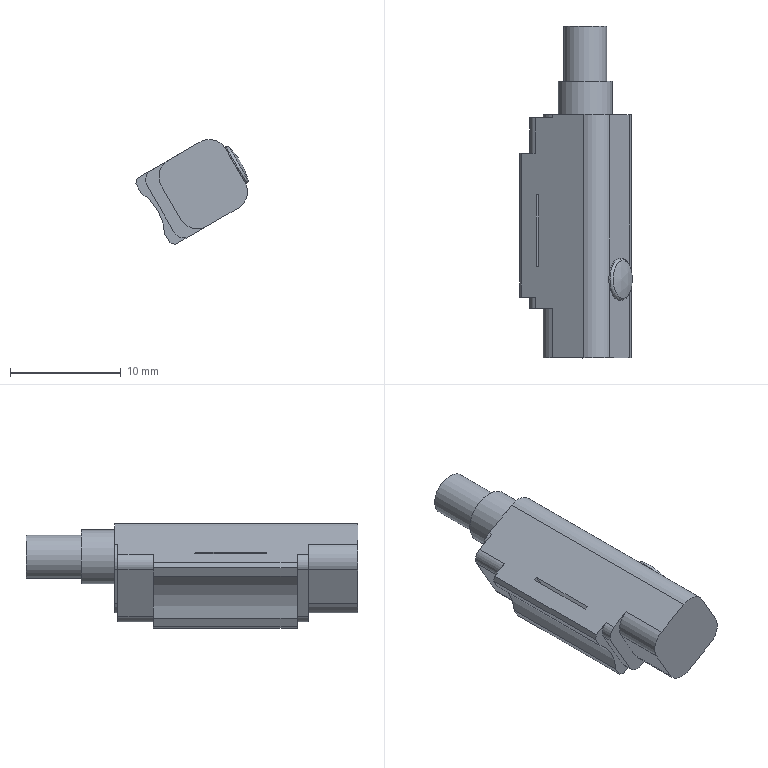Part | NX | features WGN01-25-100-Y-2-003 2 | 1 solid | 42 faces | box 10.179 x 30 x 9.481 mm | volume 1272 mm3 | plane 26 | cylinder 14 | torus 1 | sphere 1 | commonest cylinder face diameters 3.4 x6 2 x4 3.8 x1 3.9 x1 4.9 x1 10 x1
STEP:
#1=CARTESIAN_POINT('',(19.571,368.576,148.202));
#2=VERTEX_POINT('',#1);
#3=CARTESIAN_POINT('',(19.571,370.056,148.202));
#4=VERTEX_POINT('',#3);
#5=CARTESIAN_POINT('',(20.446,369.316,146.686));
#6=DIRECTION('',(-0.866,0.,-0.5));
#7=DIRECTION('',(-0.4605,-0.3894,0.7977));
#8=AXIS2_PLACEMENT_3D('',#5,#6,#7);
#9=CIRCLE('',#8,1.9);
#10=EDGE_CURVE('',#2,#4,#9,.T.);
#11=ORIENTED_EDGE('',*,*,#10,.F.);
#12=CARTESIAN_POINT('',(21.321,368.576,145.17));
#13=VERTEX_POINT('',#12);
#14=CARTESIAN_POINT('',(20.446,369.316,146.686));
#15=DIRECTION('',(-0.866,0.,-0.5));
#16=DIRECTION('',(0.4605,-0.3894,-0.7977));
#17=AXIS2_PLACEMENT_3D('',#14,#15,#16);
#18=CIRCLE('',#17,1.9);
#19=EDGE_CURVE('',#13,#2,#18,.T.);
#20=ORIENTED_EDGE('',*,*,#19,.F.);
#21=CARTESIAN_POINT('',(21.321,370.056,145.17));
#22=VERTEX_POINT('',#21);
#23=CARTESIAN_POINT('',(20.446,369.316,146.686));
#24=DIRECTION('',(-0.866,0.,-0.5));
#25=DIRECTION('',(0.4605,0.3894,-0.7977));
#26=AXIS2_PLACEMENT_3D('',#23,#24,#25);
#27=CIRCLE('',#26,1.9);
#28=EDGE_CURVE('',#22,#13,#27,.T.);
#29=ORIENTED_EDGE('',*,*,#28,.F.);
#30=CARTESIAN_POINT('',(20.446,369.316,146.686));
#31=DIRECTION('',(-0.866,0.,-0.5));
#32=DIRECTION('',(-0.4605,0.3894,0.7977));
#33=AXIS2_PLACEMENT_3D('',#30,#31,#32);
#34=CIRCLE('',#33,1.9);
#35=EDGE_CURVE('',#4,#22,#34,.T.);
#36=ORIENTED_EDGE('',*,*,#35,.F.);
#37=EDGE_LOOP('',(#11,#20,#29,#36));
#38=FACE_BOUND('',#37,.T.);
#39=CARTESIAN_POINT('',(19.596,369.316,148.389));
#40=VERTEX_POINT('',#39);
#41=CARTESIAN_POINT('',(20.546,369.316,146.744));
#42=DIRECTION('',(-0.866,0.,-0.5));
#43=DIRECTION('',(-0.5,0.,0.866));
#44=AXIS2_PLACEMENT_3D('',#41,#42,#43);
#45=CIRCLE('',#44,1.9);
#46=EDGE_CURVE('',#40,#40,#45,.T.);
#47=ORIENTED_EDGE('',*,*,#46,.T.);
#48=EDGE_LOOP('',(#47));
#49=FACE_BOUND('',#48,.T.);
#50=CARTESIAN_POINT('',(20.446,369.316,146.686));
#51=DIRECTION('',(-0.866,0.,-0.5));
#52=DIRECTION('',(0.5,0.,-0.866));
#53=AXIS2_PLACEMENT_3D('',#50,#51,#52);
#54=CYLINDRICAL_SURFACE('',#53,1.9);
#55=ADVANCED_FACE('',(#38,#49),#54,.T.);
#56=ORIENTED_EDGE('',*,*,#46,.F.);
#57=EDGE_LOOP('',(#56));
#58=FACE_BOUND('',#57,.T.);
#59=CARTESIAN_POINT('',(19.894,369.316,148.353));
#60=VERTEX_POINT('',#59);
#61=CARTESIAN_POINT('',(20.754,369.316,146.864));
#62=DIRECTION('',(-0.866,0.,-0.5));
#63=DIRECTION('',(-0.5,0.,0.866));
#64=AXIS2_PLACEMENT_3D('',#61,#62,#63);
#65=CIRCLE('',#64,1.72);
#66=EDGE_CURVE('',#60,#60,#65,.T.);
#67=ORIENTED_EDGE('',*,*,#66,.T.);
#68=EDGE_LOOP('',(#67));
#69=FACE_BOUND('',#68,.T.);
#70=CARTESIAN_POINT('',(20.546,369.316,146.744));
#71=DIRECTION('',(-0.866,0.,-0.5));
#72=DIRECTION('',(0.5,0.,-0.866));
#73=AXIS2_PLACEMENT_3D('',#70,#71,#72);
#74=TOROIDAL_SURFACE('',#73,1.65,0.25);
#75=ADVANCED_FACE('',(#58,#69),#74,.T.);
#76=ORIENTED_EDGE('',*,*,#66,.F.);
#77=EDGE_LOOP('',(#76));
#78=FACE_BOUND('',#77,.T.);
#79=CARTESIAN_POINT('',(15.623,369.316,143.901));
#80=DIRECTION('',(0.5,0.,-0.866));
#81=DIRECTION('',(0.,-1.,0.));
#82=AXIS2_PLACEMENT_3D('',#79,#80,#81);
#83=SPHERICAL_SURFACE('',#82,6.17);
#84=ADVANCED_FACE('',(#78),#83,.T.);
#85=CARTESIAN_POINT('',(18.323,387.216,144.363));
#86=VERTEX_POINT('',#85);
#87=CARTESIAN_POINT('',(17.348,387.216,146.052));
#88=DIRECTION('',(0.,-1.,0.));
#89=DIRECTION('',(0.5,0.,-0.866));
#90=AXIS2_PLACEMENT_3D('',#87,#88,#89);
#91=CIRCLE('',#90,1.95);
#92=EDGE_CURVE('',#86,#86,#91,.F.);
#93=ORIENTED_EDGE('',*,*,#92,.T.);
#94=EDGE_LOOP('',(#93));
#95=FACE_BOUND('',#94,.T.);
#96=CARTESIAN_POINT('',(18.323,392.216,144.363));
#97=VERTEX_POINT('',#96);
#98=CARTESIAN_POINT('',(17.348,392.216,146.052));
#99=DIRECTION('',(0.,-1.,0.));
#100=DIRECTION('',(0.5,0.,-0.866));
#101=AXIS2_PLACEMENT_3D('',#98,#99,#100);
#102=CIRCLE('',#101,1.95);
#103=EDGE_CURVE('',#97,#97,#102,.F.);
#104=ORIENTED_EDGE('',*,*,#103,.F.);
#105=EDGE_LOOP('',(#104));
#106=FACE_BOUND('',#105,.T.);
#107=CARTESIAN_POINT('',(17.348,392.216,146.052));
#108=DIRECTION('',(0.,-1.,0.));
#109=DIRECTION('',(-0.5,0.,0.866));
#110=AXIS2_PLACEMENT_3D('',#107,#108,#109);
#111=CYLINDRICAL_SURFACE('',#110,1.95);
#112=ADVANCED_FACE('',(#95,#106),#111,.T.);
#113=CARTESIAN_POINT('',(16.123,384.216,148.174));
#114=VERTEX_POINT('',#113);
#115=CARTESIAN_POINT('',(17.348,384.216,146.052));
#116=DIRECTION('',(0.,-1.,0.));
#117=DIRECTION('',(0.5,0.,-0.866));
#118=AXIS2_PLACEMENT_3D('',#115,#116,#117);
#119=CIRCLE('',#118,2.45);
#120=EDGE_CURVE('',#114,#114,#119,.F.);
#121=ORIENTED_EDGE('',*,*,#120,.T.);
#122=EDGE_LOOP('',(#121));
#123=FACE_BOUND('',#122,.T.);
#124=CARTESIAN_POINT('',(18.573,387.216,143.93));
#125=VERTEX_POINT('',#124);
#126=CARTESIAN_POINT('',(17.348,387.216,146.052));
#127=DIRECTION('',(0.,-1.,0.));
#128=DIRECTION('',(0.5,0.,-0.866));
#129=AXIS2_PLACEMENT_3D('',#126,#127,#128);
#130=CIRCLE('',#129,2.45);
#131=EDGE_CURVE('',#125,#125,#130,.F.);
#132=ORIENTED_EDGE('',*,*,#131,.F.);
#133=EDGE_LOOP('',(#132));
#134=FACE_BOUND('',#133,.T.);
#135=CARTESIAN_POINT('',(17.348,387.216,146.052));
#136=DIRECTION('',(0.,-1.,0.));
#137=DIRECTION('',(-0.5,0.,0.866));
#138=AXIS2_PLACEMENT_3D('',#135,#136,#137);
#139=CYLINDRICAL_SURFACE('',#138,2.45);
#140=ADVANCED_FACE('',(#123,#134),#139,.T.);
#141=CARTESIAN_POINT('',(20.699,384.216,142.848));
#142=VERTEX_POINT('',#141);
#143=CARTESIAN_POINT('',(20.699,362.216,142.848));
#144=VERTEX_POINT('',#143);
#145=CARTESIAN_POINT('',(20.699,384.216,142.848));
#146=DIRECTION('',(0.,-1.,0.));
#147=VECTOR('',#146,1000.);
#148=LINE('',#145,#147);
#149=EDGE_CURVE('',#142,#144,#148,.T.);
#150=ORIENTED_EDGE('',*,*,#149,.T.);
#151=CARTESIAN_POINT('',(17.841,362.216,141.198));
#152=VERTEX_POINT('',#151);
#153=CARTESIAN_POINT('',(20.699,362.216,142.848));
#154=DIRECTION('',(-0.866,0.,-0.5));
#155=VECTOR('',#154,1000.);
#156=LINE('',#153,#155);
#157=EDGE_CURVE('',#144,#152,#156,.T.);
#158=ORIENTED_EDGE('',*,*,#157,.T.);
#159=CARTESIAN_POINT('',(17.841,366.716,141.198));
#160=VERTEX_POINT('',#159);
#161=CARTESIAN_POINT('',(17.841,366.716,141.198));
#162=DIRECTION('',(0.,-1.,0.));
#163=VECTOR('',#162,1000.);
#164=LINE('',#161,#163);
#165=EDGE_CURVE('',#160,#152,#164,.T.);
#166=ORIENTED_EDGE('',*,*,#165,.F.);
#167=CARTESIAN_POINT('',(16.282,366.716,140.298));
#168=VERTEX_POINT('',#167);
#169=CARTESIAN_POINT('',(17.841,366.716,141.198));
#170=DIRECTION('',(-0.866,0.,-0.5));
#171=VECTOR('',#170,1000.);
#172=LINE('',#169,#171);
#173=EDGE_CURVE('',#160,#168,#172,.T.);
#174=ORIENTED_EDGE('',*,*,#173,.T.);
#175=CARTESIAN_POINT('',(16.282,367.716,140.298));
#176=VERTEX_POINT('',#175);
#177=CARTESIAN_POINT('',(16.282,367.716,140.298));
#178=DIRECTION('',(0.,-1.,0.));
#179=VECTOR('',#178,1000.);
#180=LINE('',#177,#179);
#181=EDGE_CURVE('',#176,#168,#180,.T.);
#182=ORIENTED_EDGE('',*,*,#181,.F.);
#183=CARTESIAN_POINT('',(15.021,367.716,139.57));
#184=VERTEX_POINT('',#183);
#185=CARTESIAN_POINT('',(16.282,367.716,140.298));
#186=DIRECTION('',(-0.866,0.,-0.5));
#187=VECTOR('',#186,1000.);
#188=LINE('',#185,#187);
#189=EDGE_CURVE('',#176,#184,#188,.T.);
#190=ORIENTED_EDGE('',*,*,#189,.T.);
#191=CARTESIAN_POINT('',(15.021,380.716,139.57));
#192=VERTEX_POINT('',#191);
#193=CARTESIAN_POINT('',(15.021,380.716,139.57));
#194=DIRECTION('',(0.,-1.,0.));
#195=VECTOR('',#194,1000.);
#196=LINE('',#193,#195);
#197=EDGE_CURVE('',#192,#184,#196,.T.);
#198=ORIENTED_EDGE('',*,*,#197,.F.);
#199=CARTESIAN_POINT('',(16.282,380.716,140.298));
#200=VERTEX_POINT('',#199);
#201=CARTESIAN_POINT('',(16.282,380.716,140.298));
#202=DIRECTION('',(-0.866,0.,-0.5));
#203=VECTOR('',#202,1000.);
#204=LINE('',#201,#203);
#205=EDGE_CURVE('',#200,#192,#204,.T.);
#206=ORIENTED_EDGE('',*,*,#205,.F.);
#207=CARTESIAN_POINT('',(16.282,383.916,140.298));
#208=VERTEX_POINT('',#207);
#209=CARTESIAN_POINT('',(16.282,383.916,140.298));
#210=DIRECTION('',(0.,-1.,0.));
#211=VECTOR('',#210,1000.);
#212=LINE('',#209,#211);
#213=EDGE_CURVE('',#208,#200,#212,.T.);
#214=ORIENTED_EDGE('',*,*,#213,.F.);
#215=CARTESIAN_POINT('',(17.841,383.916,141.198));
#216=VERTEX_POINT('',#215);
#217=CARTESIAN_POINT('',(17.841,383.916,141.198));
#218=DIRECTION('',(-0.866,0.,-0.5));
#219=VECTOR('',#218,1000.);
#220=LINE('',#217,#219);
#221=EDGE_CURVE('',#216,#208,#220,.T.);
#222=ORIENTED_EDGE('',*,*,#221,.F.);
#223=CARTESIAN_POINT('',(17.841,384.216,141.198));
#224=VERTEX_POINT('',#223);
#225=CARTESIAN_POINT('',(17.841,384.216,141.198));
#226=DIRECTION('',(0.,-1.,0.));
#227=VECTOR('',#226,1000.);
#228=LINE('',#225,#227);
#229=EDGE_CURVE('',#224,#216,#228,.T.);
#230=ORIENTED_EDGE('',*,*,#229,.F.);
#231=CARTESIAN_POINT('',(20.699,384.216,142.848));
#232=DIRECTION('',(-0.866,0.,-0.5));
#233=VECTOR('',#232,1000.);
#234=LINE('',#231,#233);
#235=EDGE_CURVE('',#142,#224,#234,.T.);
#236=ORIENTED_EDGE('',*,*,#235,.F.);
#237=EDGE_LOOP('',(#150,#158,#166,#174,#182,#190,#198,#206,#214,#222,#230,#236));
#238=FACE_BOUND('',#237,.T.);
#239=CARTESIAN_POINT('',(16.629,376.966,140.498));
#240=VERTEX_POINT('',#239);
#241=CARTESIAN_POINT('',(16.629,370.466,140.498));
#242=VERTEX_POINT('',#241);
#243=CARTESIAN_POINT('',(16.629,376.966,140.498));
#244=DIRECTION('',(0.,-1.,0.));
#245=VECTOR('',#244,1000.);
#246=LINE('',#243,#245);
#247=EDGE_CURVE('',#240,#242,#246,.T.);
#248=ORIENTED_EDGE('',*,*,#247,.F.);
#249=CARTESIAN_POINT('',(16.369,376.966,140.348));
#250=VERTEX_POINT('',#249);
#251=CARTESIAN_POINT('',(16.369,376.966,140.348));
#252=DIRECTION('',(0.866,0.,0.5));
#253=VECTOR('',#252,1000.);
#254=LINE('',#251,#253);
#255=EDGE_CURVE('',#250,#240,#254,.T.);
#256=ORIENTED_EDGE('',*,*,#255,.F.);
#257=CARTESIAN_POINT('',(16.369,370.466,140.348));
#258=VERTEX_POINT('',#257);
#259=CARTESIAN_POINT('',(16.369,370.466,140.348));
#260=DIRECTION('',(0.,1.,0.));
#261=VECTOR('',#260,1000.);
#262=LINE('',#259,#261);
#263=EDGE_CURVE('',#258,#250,#262,.T.);
#264=ORIENTED_EDGE('',*,*,#263,.F.);
#265=CARTESIAN_POINT('',(16.629,370.466,140.498));
#266=DIRECTION('',(-0.866,0.,-0.5));
#267=VECTOR('',#266,1000.);
#268=LINE('',#265,#267);
#269=EDGE_CURVE('',#242,#258,#268,.T.);
#270=ORIENTED_EDGE('',*,*,#269,.F.);
#271=EDGE_LOOP('',(#248,#256,#264,#270));
#272=FACE_BOUND('',#271,.T.);
#273=CARTESIAN_POINT('',(20.699,384.216,142.848));
#274=DIRECTION('',(-0.5,0.,0.866));
#275=DIRECTION('',(0.,1.,0.));
#276=AXIS2_PLACEMENT_3D('',#273,#274,#275);
#277=PLANE('',#276);
#278=ADVANCED_FACE('',(#238,#272),#277,.F.);
#279=CARTESIAN_POINT('',(14.391,384.216,147.174));
#280=VERTEX_POINT('',#279);
#281=CARTESIAN_POINT('',(14.391,383.916,147.174));
#282=VERTEX_POINT('',#281);
#283=CARTESIAN_POINT('',(14.391,384.216,147.174));
#284=DIRECTION('',(0.,-1.,0.));
#285=VECTOR('',#284,1000.);
#286=LINE('',#283,#285);
#287=EDGE_CURVE('',#280,#282,#286,.T.);
#288=ORIENTED_EDGE('',*,*,#287,.T.);
#289=CARTESIAN_POINT('',(12.832,383.916,146.274));
#290=VERTEX_POINT('',#289);
#291=CARTESIAN_POINT('',(12.832,383.916,146.274));
#292=DIRECTION('',(0.866,0.,0.5));
#293=VECTOR('',#292,1000.);
#294=LINE('',#291,#293);
#295=EDGE_CURVE('',#290,#282,#294,.T.);
#296=ORIENTED_EDGE('',*,*,#295,.F.);
#297=CARTESIAN_POINT('',(12.832,380.716,146.274));
#298=VERTEX_POINT('',#297);
#299=CARTESIAN_POINT('',(12.832,383.916,146.274));
#300=DIRECTION('',(0.,-1.,0.));
#301=VECTOR('',#300,1000.);
#302=LINE('',#299,#301);
#303=EDGE_CURVE('',#290,#298,#302,.T.);
#304=ORIENTED_EDGE('',*,*,#303,.T.);
#305=CARTESIAN_POINT('',(11.571,380.716,145.546));
#306=VERTEX_POINT('',#305);
#307=CARTESIAN_POINT('',(11.571,380.716,145.546));
#308=DIRECTION('',(0.866,0.,0.5));
#309=VECTOR('',#308,1000.);
#310=LINE('',#307,#309);
#311=EDGE_CURVE('',#306,#298,#310,.T.);
#312=ORIENTED_EDGE('',*,*,#311,.F.);
#313=CARTESIAN_POINT('',(11.571,367.716,145.546));
#314=VERTEX_POINT('',#313);
#315=CARTESIAN_POINT('',(11.571,380.716,145.546));
#316=DIRECTION('',(0.,-1.,0.));
#317=VECTOR('',#316,1000.);
#318=LINE('',#315,#317);
#319=EDGE_CURVE('',#306,#314,#318,.T.);
#320=ORIENTED_EDGE('',*,*,#319,.T.);
#321=CARTESIAN_POINT('',(12.832,367.716,146.274));
#322=VERTEX_POINT('',#321);
#323=CARTESIAN_POINT('',(11.571,367.716,145.546));
#324=DIRECTION('',(0.866,0.,0.5));
#325=VECTOR('',#324,1000.);
#326=LINE('',#323,#325);
#327=EDGE_CURVE('',#314,#322,#326,.T.);
#328=ORIENTED_EDGE('',*,*,#327,.T.);
#329=CARTESIAN_POINT('',(12.832,366.716,146.274));
#330=VERTEX_POINT('',#329);
#331=CARTESIAN_POINT('',(12.832,367.716,146.274));
#332=DIRECTION('',(0.,-1.,0.));
#333=VECTOR('',#332,1000.);
#334=LINE('',#331,#333);
#335=EDGE_CURVE('',#322,#330,#334,.T.);
#336=ORIENTED_EDGE('',*,*,#335,.T.);
#337=CARTESIAN_POINT('',(14.391,366.716,147.174));
#338=VERTEX_POINT('',#337);
#339=CARTESIAN_POINT('',(12.832,366.716,146.274));
#340=DIRECTION('',(0.866,0.,0.5));
#341=VECTOR('',#340,1000.);
#342=LINE('',#339,#341);
#343=EDGE_CURVE('',#330,#338,#342,.T.);
#344=ORIENTED_EDGE('',*,*,#343,.T.);
#345=CARTESIAN_POINT('',(14.391,362.216,147.174));
#346=VERTEX_POINT('',#345);
#347=CARTESIAN_POINT('',(14.391,366.716,147.174));
#348=DIRECTION('',(0.,-1.,0.));
#349=VECTOR('',#348,1000.);
#350=LINE('',#347,#349);
#351=EDGE_CURVE('',#338,#346,#350,.T.);
#352=ORIENTED_EDGE('',*,*,#351,.T.);
#353=CARTESIAN_POINT('',(17.249,362.216,148.824));
#354=VERTEX_POINT('',#353);
#355=CARTESIAN_POINT('',(14.391,362.216,147.174));
#356=DIRECTION('',(0.866,0.,0.5));
#357=VECTOR('',#356,1000.);
#358=LINE('',#355,#357);
#359=EDGE_CURVE('',#346,#354,#358,.T.);
#360=ORIENTED_EDGE('',*,*,#359,.T.);
#361=CARTESIAN_POINT('',(17.249,384.216,148.824));
#362=VERTEX_POINT('',#361);
#363=CARTESIAN_POINT('',(17.249,384.216,148.824));
#364=DIRECTION('',(0.,-1.,0.));
#365=VECTOR('',#364,1000.);
#366=LINE('',#363,#365);
#367=EDGE_CURVE('',#362,#354,#366,.T.);
#368=ORIENTED_EDGE('',*,*,#367,.F.);
#369=CARTESIAN_POINT('',(16.123,384.216,148.174));
#370=DIRECTION('',(0.866,0.,0.5));
#371=VECTOR('',#370,1000.);
#372=LINE('',#369,#371);
#373=EDGE_CURVE('',#114,#362,#372,.T.);
#374=ORIENTED_EDGE('',*,*,#373,.F.);
#375=CARTESIAN_POINT('',(14.391,384.216,147.174));
#376=DIRECTION('',(0.866,0.,0.5));
#377=VECTOR('',#376,1000.);
#378=LINE('',#375,#377);
#379=EDGE_CURVE('',#280,#114,#378,.T.);
#380=ORIENTED_EDGE('',*,*,#379,.F.);
#381=EDGE_LOOP('',(#288,#296,#304,#312,#320,#328,#336,#344,#352,#360,#368,#374,#380));
#382=FACE_BOUND('',#381,.T.);
#383=CARTESIAN_POINT('',(13.179,370.466,146.474));
#384=VERTEX_POINT('',#383);
#385=CARTESIAN_POINT('',(13.179,376.966,146.474));
#386=VERTEX_POINT('',#385);
#387=CARTESIAN_POINT('',(13.179,370.466,146.474));
#388=DIRECTION('',(0.,1.,0.));
#389=VECTOR('',#388,1000.);
#390=LINE('',#387,#389);
#391=EDGE_CURVE('',#384,#386,#390,.T.);
#392=ORIENTED_EDGE('',*,*,#391,.F.);
#393=CARTESIAN_POINT('',(12.919,370.466,146.324));
#394=VERTEX_POINT('',#393);
#395=CARTESIAN_POINT('',(12.919,370.466,146.324));
#396=DIRECTION('',(0.866,0.,0.5));
#397=VECTOR('',#396,1000.);
#398=LINE('',#395,#397);
#399=EDGE_CURVE('',#394,#384,#398,.T.);
#400=ORIENTED_EDGE('',*,*,#399,.F.);
#401=CARTESIAN_POINT('',(12.919,376.966,146.324));
#402=VERTEX_POINT('',#401);
#403=CARTESIAN_POINT('',(12.919,376.966,146.324));
#404=DIRECTION('',(0.,-1.,0.));
#405=VECTOR('',#404,1000.);
#406=LINE('',#403,#405);
#407=EDGE_CURVE('',#402,#394,#406,.T.);
#408=ORIENTED_EDGE('',*,*,#407,.F.);
#409=CARTESIAN_POINT('',(13.179,376.966,146.474));
#410=DIRECTION('',(-0.866,0.,-0.5));
#411=VECTOR('',#410,1000.);
#412=LINE('',#409,#411);
#413=EDGE_CURVE('',#386,#402,#412,.T.);
#414=ORIENTED_EDGE('',*,*,#413,.F.);
#415=EDGE_LOOP('',(#392,#400,#408,#414));
#416=FACE_BOUND('',#415,.T.);
#417=CARTESIAN_POINT('',(14.391,384.216,147.174));
#418=DIRECTION('',(0.5,0.,-0.866));
#419=DIRECTION('',(0.,-1.,0.));
#420=AXIS2_PLACEMENT_3D('',#417,#418,#419);
#421=PLANE('',#420);
#422=ADVANCED_FACE('',(#382,#416),#421,.F.);
#423=ORIENTED_EDGE('',*,*,#19,.T.);
#424=CARTESIAN_POINT('',(19.571,362.216,148.202));
#425=VERTEX_POINT('',#424);
#426=CARTESIAN_POINT('',(19.571,368.576,148.202));
#427=DIRECTION('',(0.,-1.,0.));
#428=VECTOR('',#427,1000.);
#429=LINE('',#426,#428);
#430=EDGE_CURVE('',#2,#425,#429,.T.);
#431=ORIENTED_EDGE('',*,*,#430,.T.);
#432=CARTESIAN_POINT('',(21.321,362.216,145.17));
#433=VERTEX_POINT('',#432);
#434=CARTESIAN_POINT('',(19.571,362.216,148.202));
#435=DIRECTION('',(0.5,0.,-0.866));
#436=VECTOR('',#435,1000.);
#437=LINE('',#434,#436);
#438=EDGE_CURVE('',#425,#433,#437,.T.);
#439=ORIENTED_EDGE('',*,*,#438,.T.);
#440=CARTESIAN_POINT('',(21.321,368.576,145.17));
#441=DIRECTION('',(0.,-1.,0.));
#442=VECTOR('',#441,1000.);
#443=LINE('',#440,#442);
#444=EDGE_CURVE('',#13,#433,#443,.T.);
#445=ORIENTED_EDGE('',*,*,#444,.F.);
#446=EDGE_LOOP('',(#423,#431,#439,#445));
#447=FACE_BOUND('',#446,.T.);
#448=CARTESIAN_POINT('',(19.571,384.216,148.202));
#449=DIRECTION('',(-0.866,0.,-0.5));
#450=DIRECTION('',(0.5,0.,-0.866));
#451=AXIS2_PLACEMENT_3D('',#448,#449,#450);
#452=PLANE('',#451);
#453=ADVANCED_FACE('',(#447),#452,.F.);
#454=CARTESIAN_POINT('',(14.916,367.716,140.664));
#455=VERTEX_POINT('',#454);
#456=CARTESIAN_POINT('',(15.782,367.716,141.164));
#457=DIRECTION('',(0.,1.,0.));
#458=DIRECTION('',(0.5,0.,-0.866));
#459=AXIS2_PLACEMENT_3D('',#456,#457,#458);
#460=CIRCLE('',#459,1.);
#461=EDGE_CURVE('',#176,#455,#460,.T.);
#462=ORIENTED_EDGE('',*,*,#461,.F.);
#463=ORIENTED_EDGE('',*,*,#181,.T.);
#464=CARTESIAN_POINT('',(14.916,366.716,140.664));
#465=VERTEX_POINT('',#464);
#466=CARTESIAN_POINT('',(15.782,366.716,141.164));
#467=DIRECTION('',(0.,1.,0.));
#468=DIRECTION('',(0.5,0.,-0.866));
#469=AXIS2_PLACEMENT_3D('',#466,#467,#468);
#470=CIRCLE('',#469,1.);
#471=EDGE_CURVE('',#168,#465,#470,.T.);
#472=ORIENTED_EDGE('',*,*,#471,.T.);
#473=CARTESIAN_POINT('',(14.916,367.716,140.664));
#474=DIRECTION('',(0.,-1.,0.));
#475=VECTOR('',#474,1000.);
#476=LINE('',#473,#475);
#477=EDGE_CURVE('',#455,#465,#476,.T.);
#478=ORIENTED_EDGE('',*,*,#477,.F.);
#479=EDGE_LOOP('',(#462,#463,#472,#478));
#480=FACE_BOUND('',#479,.T.);
#481=CARTESIAN_POINT('',(15.782,383.916,141.164));
#482=DIRECTION('',(0.,-1.,0.));
#483=DIRECTION('',(-0.5,0.,0.866));
#484=AXIS2_PLACEMENT_3D('',#481,#482,#483);
#485=CYLINDRICAL_SURFACE('',#484,1.);
#486=ADVANCED_FACE('',(#480),#485,.T.);
#487=CARTESIAN_POINT('',(12.466,367.716,144.908));
#488=VERTEX_POINT('',#487);
#489=CARTESIAN_POINT('',(12.466,367.716,144.908));
#490=DIRECTION('',(0.5,0.,-0.866));
#491=VECTOR('',#490,1000.);
#492=LINE('',#489,#491);
#493=EDGE_CURVE('',#488,#455,#492,.T.);
#494=ORIENTED_EDGE('',*,*,#493,.T.);
#495=ORIENTED_EDGE('',*,*,#477,.T.);
#496=CARTESIAN_POINT('',(12.466,366.716,144.908));
#497=VERTEX_POINT('',#496);
#498=CARTESIAN_POINT('',(14.916,366.716,140.664));
#499=DIRECTION('',(-0.5,0.,0.866));
#500=VECTOR('',#499,1000.);
#501=LINE('',#498,#500);
#502=EDGE_CURVE('',#465,#497,#501,.T.);
#503=ORIENTED_EDGE('',*,*,#502,.T.);
#504=CARTESIAN_POINT('',(12.466,367.716,144.908));
#505=DIRECTION('',(0.,-1.,0.));
#506=VECTOR('',#505,1000.);
#507=LINE('',#504,#506);
#508=EDGE_CURVE('',#488,#497,#507,.T.);
#509=ORIENTED_EDGE('',*,*,#508,.F.);
#510=EDGE_LOOP('',(#494,#495,#503,#509));
#511=FACE_BOUND('',#510,.T.);
#512=CARTESIAN_POINT('',(14.916,383.916,140.664));
#513=DIRECTION('',(0.866,0.,0.5));
#514=DIRECTION('',(-0.5,0.,0.866));
#515=AXIS2_PLACEMENT_3D('',#512,#513,#514);
#516=PLANE('',#515);
#517=ADVANCED_FACE('',(#511),#516,.F.);
#518=ORIENTED_EDGE('',*,*,#335,.F.);
#519=CARTESIAN_POINT('',(13.332,367.716,145.408));
#520=DIRECTION('',(0.,1.,0.));
#521=DIRECTION('',(-0.866,0.,-0.5));
#522=AXIS2_PLACEMENT_3D('',#519,#520,#521);
#523=CIRCLE('',#522,1.);
#524=EDGE_CURVE('',#488,#322,#523,.T.);
#525=ORIENTED_EDGE('',*,*,#524,.F.);
#526=ORIENTED_EDGE('',*,*,#508,.T.);
#527=CARTESIAN_POINT('',(13.332,366.716,145.408));
#528=DIRECTION('',(0.,1.,0.));
#529=DIRECTION('',(-0.866,0.,-0.5));
#530=AXIS2_PLACEMENT_3D('',#527,#528,#529);
#531=CIRCLE('',#530,1.);
#532=EDGE_CURVE('',#497,#330,#531,.T.);
#533=ORIENTED_EDGE('',*,*,#532,.T.);
#534=EDGE_LOOP('',(#518,#525,#526,#533));
#535=FACE_BOUND('',#534,.T.);
#536=CARTESIAN_POINT('',(13.332,383.916,145.408));
#537=DIRECTION('',(0.,-1.,0.));
#538=DIRECTION('',(-0.5,0.,0.866));
#539=AXIS2_PLACEMENT_3D('',#536,#537,#538);
#540=CYLINDRICAL_SURFACE('',#539,1.);
#541=ADVANCED_FACE('',(#535),#540,.T.);
#542=CARTESIAN_POINT('',(15.519,366.716,141.82));
#543=VERTEX_POINT('',#542);
#544=CARTESIAN_POINT('',(16.991,366.716,142.67));
#545=DIRECTION('',(0.,1.,0.));
#546=DIRECTION('',(0.5,0.,-0.866));
#547=AXIS2_PLACEMENT_3D('',#544,#545,#546);
#548=CIRCLE('',#547,1.7);
#549=EDGE_CURVE('',#160,#543,#548,.T.);
#550=ORIENTED_EDGE('',*,*,#549,.F.);
#551=ORIENTED_EDGE('',*,*,#165,.T.);
#552=CARTESIAN_POINT('',(15.519,362.216,141.82));
#553=VERTEX_POINT('',#552);
#554=CARTESIAN_POINT('',(16.991,362.216,142.67));
#555=DIRECTION('',(0.,1.,0.));
#556=DIRECTION('',(0.5,0.,-0.866));
#557=AXIS2_PLACEMENT_3D('',#554,#555,#556);
#558=CIRCLE('',#557,1.7);
#559=EDGE_CURVE('',#152,#553,#558,.T.);
#560=ORIENTED_EDGE('',*,*,#559,.T.);
#561=CARTESIAN_POINT('',(15.519,366.716,141.82));
#562=DIRECTION('',(0.,-1.,0.));
#563=VECTOR('',#562,1000.);
#564=LINE('',#561,#563);
#565=EDGE_CURVE('',#543,#553,#564,.T.);
#566=ORIENTED_EDGE('',*,*,#565,.F.);
#567=EDGE_LOOP('',(#550,#551,#560,#566));
#568=FACE_BOUND('',#567,.T.);
#569=CARTESIAN_POINT('',(16.991,384.216,142.67));
#570=DIRECTION('',(0.,-1.,0.));
#571=DIRECTION('',(-0.5,0.,0.866));
#572=AXIS2_PLACEMENT_3D('',#569,#570,#571);
#573=CYLINDRICAL_SURFACE('',#572,1.7);
#574=ADVANCED_FACE('',(#568),#573,.T.);
#575=CARTESIAN_POINT('',(13.769,366.716,144.852));
#576=VERTEX_POINT('',#575);
#577=CARTESIAN_POINT('',(15.519,366.716,141.82));
#578=DIRECTION('',(-0.5,0.,0.866));
#579=VECTOR('',#578,1000.);
#580=LINE('',#577,#579);
#581=EDGE_CURVE('',#543,#576,#580,.T.);
#582=ORIENTED_EDGE('',*,*,#581,.F.);
#583=ORIENTED_EDGE('',*,*,#565,.T.);
#584=CARTESIAN_POINT('',(13.769,362.216,144.852));
#585=VERTEX_POINT('',#584);
#586=CARTESIAN_POINT('',(15.519,362.216,141.82));
#587=DIRECTION('',(-0.5,0.,0.866));
#588=VECTOR('',#587,1000.);
#589=LINE('',#586,#588);
#590=EDGE_CURVE('',#553,#585,#589,.T.);
#591=ORIENTED_EDGE('',*,*,#590,.T.);
#592=CARTESIAN_POINT('',(13.769,366.716,144.852));
#593=DIRECTION('',(0.,-1.,0.));
#594=VECTOR('',#593,1000.);
#595=LINE('',#592,#594);
#596=EDGE_CURVE('',#576,#585,#595,.T.);
#597=ORIENTED_EDGE('',*,*,#596,.F.);
#598=EDGE_LOOP('',(#582,#583,#591,#597));
#599=FACE_BOUND('',#598,.T.);
#600=CARTESIAN_POINT('',(15.519,384.216,141.82));
#601=DIRECTION('',(0.866,0.,0.5));
#602=DIRECTION('',(-0.5,0.,0.866));
#603=AXIS2_PLACEMENT_3D('',#600,#601,#602);
#604=PLANE('',#603);
#605=ADVANCED_FACE('',(#599),#604,.F.);
#606=CARTESIAN_POINT('',(15.241,366.716,145.702));
#607=DIRECTION('',(0.,1.,0.));
#608=DIRECTION('',(-0.866,0.,-0.5));
#609=AXIS2_PLACEMENT_3D('',#606,#607,#608);
#610=CIRCLE('',#609,1.7);
#611=EDGE_CURVE('',#576,#338,#610,.T.);
#612=ORIENTED_EDGE('',*,*,#611,.F.);
#613=ORIENTED_EDGE('',*,*,#596,.T.);
#614=CARTESIAN_POINT('',(15.241,362.216,145.702));
#615=DIRECTION('',(0.,1.,0.));
#616=DIRECTION('',(-0.866,0.,-0.5));
#617=AXIS2_PLACEMENT_3D('',#614,#615,#616);
#618=CIRCLE('',#617,1.7);
#619=EDGE_CURVE('',#585,#346,#618,.T.);
#620=ORIENTED_EDGE('',*,*,#619,.T.);
#621=ORIENTED_EDGE('',*,*,#351,.F.);
#622=EDGE_LOOP('',(#612,#613,#620,#621));
#623=FACE_BOUND('',#622,.T.);
#624=CARTESIAN_POINT('',(15.241,384.216,145.702));
#625=DIRECTION('',(0.,-1.,0.));
#626=DIRECTION('',(-0.5,0.,0.866));
#627=AXIS2_PLACEMENT_3D('',#624,#625,#626);
#628=CYLINDRICAL_SURFACE('',#627,1.7);
#629=ADVANCED_FACE('',(#623),#628,.T.);
#630=ORIENTED_EDGE('',*,*,#229,.T.);
#631=CARTESIAN_POINT('',(15.519,383.916,141.82));
#632=VERTEX_POINT('',#631);
#633=CARTESIAN_POINT('',(16.991,383.916,142.67));
#634=DIRECTION('',(0.,1.,0.));
#635=DIRECTION('',(0.5,0.,-0.866));
#636=AXIS2_PLACEMENT_3D('',#633,#634,#635);
#637=CIRCLE('',#636,1.7);
#638=EDGE_CURVE('',#216,#632,#637,.T.);
#639=ORIENTED_EDGE('',*,*,#638,.T.);
#640=CARTESIAN_POINT('',(15.519,384.216,141.82));
#641=VERTEX_POINT('',#640);
#642=CARTESIAN_POINT('',(15.519,384.216,141.82));
#643=DIRECTION('',(0.,-1.,0.));
#644=VECTOR('',#643,1000.);
#645=LINE('',#642,#644);
#646=EDGE_CURVE('',#641,#632,#645,.T.);
#647=ORIENTED_EDGE('',*,*,#646,.F.);
#648=CARTESIAN_POINT('',(16.991,384.216,142.67));
#649=DIRECTION('',(0.,1.,0.));
#650=DIRECTION('',(0.5,0.,-0.866));
#651=AXIS2_PLACEMENT_3D('',#648,#649,#650);
#652=CIRCLE('',#651,1.7);
#653=EDGE_CURVE('',#224,#641,#652,.T.);
#654=ORIENTED_EDGE('',*,*,#653,.F.);
#655=EDGE_LOOP('',(#630,#639,#647,#654));
#656=FACE_BOUND('',#655,.T.);
#657=CARTESIAN_POINT('',(16.991,384.216,142.67));
#658=DIRECTION('',(0.,-1.,0.));
#659=DIRECTION('',(-0.5,0.,0.866));
#660=AXIS2_PLACEMENT_3D('',#657,#658,#659);
#661=CYLINDRICAL_SURFACE('',#660,1.7);
#662=ADVANCED_FACE('',(#656),#661,.T.);
#663=ORIENTED_EDGE('',*,*,#646,.T.);
#664=CARTESIAN_POINT('',(13.769,383.916,144.852));
#665=VERTEX_POINT('',#664);
#666=CARTESIAN_POINT('',(15.519,383.916,141.82));
#667=DIRECTION('',(-0.5,0.,0.866));
#668=VECTOR('',#667,1000.);
#669=LINE('',#666,#668);
#670=EDGE_CURVE('',#632,#665,#669,.T.);
#671=ORIENTED_EDGE('',*,*,#670,.T.);
#672=CARTESIAN_POINT('',(13.769,384.216,144.852));
#673=VERTEX_POINT('',#672);
#674=CARTESIAN_POINT('',(13.769,384.216,144.852));
#675=DIRECTION('',(0.,-1.,0.));
#676=VECTOR('',#675,1000.);
#677=LINE('',#674,#676);
#678=EDGE_CURVE('',#673,#665,#677,.T.);
#679=ORIENTED_EDGE('',*,*,#678,.F.);
#680=CARTESIAN_POINT('',(15.519,384.216,141.82));
#681=DIRECTION('',(-0.5,0.,0.866));
#682=VECTOR('',#681,1000.);
#683=LINE('',#680,#682);
#684=EDGE_CURVE('',#641,#673,#683,.T.);
#685=ORIENTED_EDGE('',*,*,#684,.F.);
#686=EDGE_LOOP('',(#663,#671,#679,#685));
#687=FACE_BOUND('',#686,.T.);
#688=CARTESIAN_POINT('',(15.519,384.216,141.82));
#689=DIRECTION('',(0.866,0.,0.5));
#690=DIRECTION('',(-0.5,0.,0.866));
#691=AXIS2_PLACEMENT_3D('',#688,#689,#690);
#692=PLANE('',#691);
#693=ADVANCED_FACE('',(#687),#692,.F.);
#694=ORIENTED_EDGE('',*,*,#678,.T.);
#695=CARTESIAN_POINT('',(15.241,383.916,145.702));
#696=DIRECTION('',(0.,1.,0.));
#697=DIRECTION('',(-0.866,0.,-0.5));
#698=AXIS2_PLACEMENT_3D('',#695,#696,#697);
#699=CIRCLE('',#698,1.7);
#700=EDGE_CURVE('',#665,#282,#699,.T.);
#701=ORIENTED_EDGE('',*,*,#700,.T.);
#702=ORIENTED_EDGE('',*,*,#287,.F.);
#703=CARTESIAN_POINT('',(15.241,384.216,145.702));
#704=DIRECTION('',(0.,1.,0.));
#705=DIRECTION('',(-0.866,0.,-0.5));
#706=AXIS2_PLACEMENT_3D('',#703,#704,#705);
#707=CIRCLE('',#706,1.7);
#708=EDGE_CURVE('',#673,#280,#707,.T.);
#709=ORIENTED_EDGE('',*,*,#708,.F.);
#710=EDGE_LOOP('',(#694,#701,#702,#709));
#711=FACE_BOUND('',#710,.T.);
#712=CARTESIAN_POINT('',(15.241,384.216,145.702));
#713=DIRECTION('',(0.,-1.,0.));
#714=DIRECTION('',(-0.5,0.,0.866));
#715=AXIS2_PLACEMENT_3D('',#712,#713,#714);
#716=CYLINDRICAL_SURFACE('',#715,1.7);
#717=ADVANCED_FACE('',(#711),#716,.T.);
#718=ORIENTED_EDGE('',*,*,#367,.T.);
#719=CARTESIAN_POINT('',(18.099,362.216,147.352));
#720=DIRECTION('',(0.,1.,0.));
#721=DIRECTION('',(-0.5,0.,0.866));
#722=AXIS2_PLACEMENT_3D('',#719,#720,#721);
#723=CIRCLE('',#722,1.7);
#724=EDGE_CURVE('',#354,#425,#723,.T.);
#725=ORIENTED_EDGE('',*,*,#724,.T.);
#726=ORIENTED_EDGE('',*,*,#430,.F.);
#727=CARTESIAN_POINT('',(19.571,370.056,148.202));
#728=DIRECTION('',(0.,-1.,0.));
#729=VECTOR('',#728,1000.);
#730=LINE('',#727,#729);
#731=EDGE_CURVE('',#4,#2,#730,.T.);
#732=ORIENTED_EDGE('',*,*,#731,.F.);
#733=CARTESIAN_POINT('',(19.571,384.216,148.202));
#734=VERTEX_POINT('',#733);
#735=CARTESIAN_POINT('',(19.571,384.216,148.202));
#736=DIRECTION('',(0.,-1.,0.));
#737=VECTOR('',#736,1000.);
#738=LINE('',#735,#737);
#739=EDGE_CURVE('',#734,#4,#738,.T.);
#740=ORIENTED_EDGE('',*,*,#739,.F.);
#741=CARTESIAN_POINT('',(18.099,384.216,147.352));
#742=DIRECTION('',(0.,1.,0.));
#743=DIRECTION('',(-0.5,0.,0.866));
#744=AXIS2_PLACEMENT_3D('',#741,#742,#743);
#745=CIRCLE('',#744,1.7);
#746=EDGE_CURVE('',#362,#734,#745,.T.);
#747=ORIENTED_EDGE('',*,*,#746,.F.);
#748=EDGE_LOOP('',(#718,#725,#726,#732,#740,#747));
#749=FACE_BOUND('',#748,.T.);
#750=CARTESIAN_POINT('',(18.099,384.216,147.352));
#751=DIRECTION('',(0.,-1.,0.));
#752=DIRECTION('',(-0.5,0.,0.866));
#753=AXIS2_PLACEMENT_3D('',#750,#751,#752);
#754=CYLINDRICAL_SURFACE('',#753,1.7);
#755=ADVANCED_FACE('',(#749),#754,.T.);
#756=ORIENTED_EDGE('',*,*,#35,.T.);
#757=CARTESIAN_POINT('',(21.321,384.216,145.17));
#758=VERTEX_POINT('',#757);
#759=CARTESIAN_POINT('',(21.321,384.216,145.17));
#760=DIRECTION('',(0.,-1.,0.));
#761=VECTOR('',#760,1000.);
#762=LINE('',#759,#761);
#763=EDGE_CURVE('',#758,#22,#762,.T.);
#764=ORIENTED_EDGE('',*,*,#763,.F.);
#765=CARTESIAN_POINT('',(19.571,384.216,148.202));
#766=DIRECTION('',(0.5,0.,-0.866));
#767=VECTOR('',#766,1000.);
#768=LINE('',#765,#767);
#769=EDGE_CURVE('',#734,#758,#768,.T.);
#770=ORIENTED_EDGE('',*,*,#769,.F.);
#771=ORIENTED_EDGE('',*,*,#739,.T.);
#772=EDGE_LOOP('',(#756,#764,#770,#771));
#773=FACE_BOUND('',#772,.T.);
#774=CARTESIAN_POINT('',(19.571,384.216,148.202));
#775=DIRECTION('',(-0.866,0.,-0.5));
#776=DIRECTION('',(0.5,0.,-0.866));
#777=AXIS2_PLACEMENT_3D('',#774,#775,#776);
#778=PLANE('',#777);
#779=ADVANCED_FACE('',(#773),#778,.F.);
#780=ORIENTED_EDGE('',*,*,#763,.T.);
#781=CARTESIAN_POINT('',(21.321,370.056,145.17));
#782=DIRECTION('',(0.,-1.,0.));
#783=VECTOR('',#782,1000.);
#784=LINE('',#781,#783);
#785=EDGE_CURVE('',#22,#13,#784,.T.);
#786=ORIENTED_EDGE('',*,*,#785,.T.);
#787=ORIENTED_EDGE('',*,*,#444,.T.);
#788=CARTESIAN_POINT('',(19.849,362.216,144.32));
#789=DIRECTION('',(0.,1.,0.));
#790=DIRECTION('',(0.866,0.,0.5));
#791=AXIS2_PLACEMENT_3D('',#788,#789,#790);
#792=CIRCLE('',#791,1.7);
#793=EDGE_CURVE('',#433,#144,#792,.T.);
#794=ORIENTED_EDGE('',*,*,#793,.T.);
#795=ORIENTED_EDGE('',*,*,#149,.F.);
#796=CARTESIAN_POINT('',(19.849,384.216,144.32));
#797=DIRECTION('',(0.,1.,0.));
#798=DIRECTION('',(0.866,0.,0.5));
#799=AXIS2_PLACEMENT_3D('',#796,#797,#798);
#800=CIRCLE('',#799,1.7);
#801=EDGE_CURVE('',#758,#142,#800,.T.);
#802=ORIENTED_EDGE('',*,*,#801,.F.);
#803=EDGE_LOOP('',(#780,#786,#787,#794,#795,#802));
#804=FACE_BOUND('',#803,.T.);
#805=CARTESIAN_POINT('',(19.849,384.216,144.32));
#806=DIRECTION('',(0.,-1.,0.));
#807=DIRECTION('',(-0.5,0.,0.866));
#808=AXIS2_PLACEMENT_3D('',#805,#806,#807);
#809=CYLINDRICAL_SURFACE('',#808,1.7);
#810=ADVANCED_FACE('',(#804),#809,.T.);
#811=ORIENTED_EDGE('',*,*,#379,.T.);
#812=ORIENTED_EDGE('',*,*,#120,.F.);
#813=ORIENTED_EDGE('',*,*,#373,.T.);
#814=ORIENTED_EDGE('',*,*,#746,.T.);
#815=ORIENTED_EDGE('',*,*,#769,.T.);
#816=ORIENTED_EDGE('',*,*,#801,.T.);
#817=ORIENTED_EDGE('',*,*,#235,.T.);
#818=ORIENTED_EDGE('',*,*,#653,.T.);
#819=ORIENTED_EDGE('',*,*,#684,.T.);
#820=ORIENTED_EDGE('',*,*,#708,.T.);
#821=EDGE_LOOP('',(#811,#812,#813,#814,#815,#816,#817,#818,#819,#820));
#822=FACE_BOUND('',#821,.T.);
#823=CARTESIAN_POINT('',(16.991,384.216,142.67));
#824=DIRECTION('',(0.,1.,0.));
#825=DIRECTION('',(0.5,0.,-0.866));
#826=AXIS2_PLACEMENT_3D('',#823,#824,#825);
#827=PLANE('',#826);
#828=ADVANCED_FACE('',(#822),#827,.T.);
#829=ORIENTED_EDGE('',*,*,#157,.F.);
#830=ORIENTED_EDGE('',*,*,#793,.F.);
#831=ORIENTED_EDGE('',*,*,#438,.F.);
#832=ORIENTED_EDGE('',*,*,#724,.F.);
#833=ORIENTED_EDGE('',*,*,#359,.F.);
#834=ORIENTED_EDGE('',*,*,#619,.F.);
#835=ORIENTED_EDGE('',*,*,#590,.F.);
#836=ORIENTED_EDGE('',*,*,#559,.F.);
#837=EDGE_LOOP('',(#829,#830,#831,#832,#833,#834,#835,#836));
#838=FACE_BOUND('',#837,.T.);
#839=CARTESIAN_POINT('',(16.991,362.216,142.67));
#840=DIRECTION('',(0.,1.,0.));
#841=DIRECTION('',(0.5,0.,-0.866));
#842=AXIS2_PLACEMENT_3D('',#839,#840,#841);
#843=PLANE('',#842);
#844=ADVANCED_FACE('',(#838),#843,.F.);
#845=ORIENTED_EDGE('',*,*,#213,.T.);
#846=CARTESIAN_POINT('',(14.916,380.716,140.664));
#847=VERTEX_POINT('',#846);
#848=CARTESIAN_POINT('',(15.782,380.716,141.164));
#849=DIRECTION('',(0.,1.,0.));
#850=DIRECTION('',(0.5,0.,-0.866));
#851=AXIS2_PLACEMENT_3D('',#848,#849,#850);
#852=CIRCLE('',#851,1.);
#853=EDGE_CURVE('',#200,#847,#852,.T.);
#854=ORIENTED_EDGE('',*,*,#853,.T.);
#855=CARTESIAN_POINT('',(14.916,383.916,140.664));
#856=VERTEX_POINT('',#855);
#857=CARTESIAN_POINT('',(14.916,383.916,140.664));
#858=DIRECTION('',(0.,-1.,0.));
#859=VECTOR('',#858,1000.);
#860=LINE('',#857,#859);
#861=EDGE_CURVE('',#856,#847,#860,.T.);
#862=ORIENTED_EDGE('',*,*,#861,.F.);
#863=CARTESIAN_POINT('',(15.782,383.916,141.164));
#864=DIRECTION('',(0.,1.,0.));
#865=DIRECTION('',(0.5,0.,-0.866));
#866=AXIS2_PLACEMENT_3D('',#863,#864,#865);
#867=CIRCLE('',#866,1.);
#868=EDGE_CURVE('',#208,#856,#867,.T.);
#869=ORIENTED_EDGE('',*,*,#868,.F.);
#870=EDGE_LOOP('',(#845,#854,#862,#869));
#871=FACE_BOUND('',#870,.T.);
#872=CARTESIAN_POINT('',(15.782,383.916,141.164));
#873=DIRECTION('',(0.,-1.,0.));
#874=DIRECTION('',(-0.5,0.,0.866));
#875=AXIS2_PLACEMENT_3D('',#872,#873,#874);
#876=CYLINDRICAL_SURFACE('',#875,1.);
#877=ADVANCED_FACE('',(#871),#876,.T.);
#878=ORIENTED_EDGE('',*,*,#861,.T.);
#879=CARTESIAN_POINT('',(12.466,380.716,144.908));
#880=VERTEX_POINT('',#879);
#881=CARTESIAN_POINT('',(12.466,380.716,144.908));
#882=DIRECTION('',(0.5,0.,-0.866));
#883=VECTOR('',#882,1000.);
#884=LINE('',#881,#883);
#885=EDGE_CURVE('',#880,#847,#884,.T.);
#886=ORIENTED_EDGE('',*,*,#885,.F.);
#887=CARTESIAN_POINT('',(12.466,383.916,144.908));
#888=VERTEX_POINT('',#887);
#889=CARTESIAN_POINT('',(12.466,383.916,144.908));
#890=DIRECTION('',(0.,-1.,0.));
#891=VECTOR('',#890,1000.);
#892=LINE('',#889,#891);
#893=EDGE_CURVE('',#888,#880,#892,.T.);
#894=ORIENTED_EDGE('',*,*,#893,.F.);
#895=CARTESIAN_POINT('',(14.916,383.916,140.664));
#896=DIRECTION('',(-0.5,0.,0.866));
#897=VECTOR('',#896,1000.);
#898=LINE('',#895,#897);
#899=EDGE_CURVE('',#856,#888,#898,.T.);
#900=ORIENTED_EDGE('',*,*,#899,.F.);
#901=EDGE_LOOP('',(#878,#886,#894,#900));
#902=FACE_BOUND('',#901,.T.);
#903=CARTESIAN_POINT('',(14.916,383.916,140.664));
#904=DIRECTION('',(0.866,0.,0.5));
#905=DIRECTION('',(-0.5,0.,0.866));
#906=AXIS2_PLACEMENT_3D('',#903,#904,#905);
#907=PLANE('',#906);
#908=ADVANCED_FACE('',(#902),#907,.F.);
#909=ORIENTED_EDGE('',*,*,#893,.T.);
#910=CARTESIAN_POINT('',(13.332,380.716,145.408));
#911=DIRECTION('',(0.,1.,0.));
#912=DIRECTION('',(-0.866,0.,-0.5));
#913=AXIS2_PLACEMENT_3D('',#910,#911,#912);
#914=CIRCLE('',#913,1.);
#915=EDGE_CURVE('',#880,#298,#914,.T.);
#916=ORIENTED_EDGE('',*,*,#915,.T.);
#917=ORIENTED_EDGE('',*,*,#303,.F.);
#918=CARTESIAN_POINT('',(13.332,383.916,145.408));
#919=DIRECTION('',(0.,1.,0.));
#920=DIRECTION('',(-0.866,0.,-0.5));
#921=AXIS2_PLACEMENT_3D('',#918,#919,#920);
#922=CIRCLE('',#921,1.);
#923=EDGE_CURVE('',#888,#290,#922,.T.);
#924=ORIENTED_EDGE('',*,*,#923,.F.);
#925=EDGE_LOOP('',(#909,#916,#917,#924));
#926=FACE_BOUND('',#925,.T.);
#927=CARTESIAN_POINT('',(13.332,383.916,145.408));
#928=DIRECTION('',(0.,-1.,0.));
#929=DIRECTION('',(-0.5,0.,0.866));
#930=AXIS2_PLACEMENT_3D('',#927,#928,#929);
#931=CYLINDRICAL_SURFACE('',#930,1.);
#932=ADVANCED_FACE('',(#926),#931,.T.);
#933=ORIENTED_EDGE('',*,*,#638,.F.);
#934=ORIENTED_EDGE('',*,*,#221,.T.);
#935=ORIENTED_EDGE('',*,*,#868,.T.);
#936=ORIENTED_EDGE('',*,*,#899,.T.);
#937=ORIENTED_EDGE('',*,*,#923,.T.);
#938=ORIENTED_EDGE('',*,*,#295,.T.);
#939=ORIENTED_EDGE('',*,*,#700,.F.);
#940=ORIENTED_EDGE('',*,*,#670,.F.);
#941=EDGE_LOOP('',(#933,#934,#935,#936,#937,#938,#939,#940));
#942=FACE_BOUND('',#941,.T.);
#943=CARTESIAN_POINT('',(15.782,383.916,141.164));
#944=DIRECTION('',(0.,1.,0.));
#945=DIRECTION('',(0.5,0.,-0.866));
#946=AXIS2_PLACEMENT_3D('',#943,#944,#945);
#947=PLANE('',#946);
#948=ADVANCED_FACE('',(#942),#947,.T.);
#949=ORIENTED_EDGE('',*,*,#173,.F.);
#950=ORIENTED_EDGE('',*,*,#549,.T.);
#951=ORIENTED_EDGE('',*,*,#581,.T.);
#952=ORIENTED_EDGE('',*,*,#611,.T.);
#953=ORIENTED_EDGE('',*,*,#343,.F.);
#954=ORIENTED_EDGE('',*,*,#532,.F.);
#955=ORIENTED_EDGE('',*,*,#502,.F.);
#956=ORIENTED_EDGE('',*,*,#471,.F.);
#957=EDGE_LOOP('',(#949,#950,#951,#952,#953,#954,#955,#956));
#958=FACE_BOUND('',#957,.T.);
#959=CARTESIAN_POINT('',(15.782,366.716,141.164));
#960=DIRECTION('',(0.,1.,0.));
#961=DIRECTION('',(0.5,0.,-0.866));
#962=AXIS2_PLACEMENT_3D('',#959,#960,#961);
#963=PLANE('',#962);
#964=ADVANCED_FACE('',(#958),#963,.F.);
#965=CARTESIAN_POINT('',(11.442,367.716,145.063));
#966=VERTEX_POINT('',#965);
#967=CARTESIAN_POINT('',(11.442,367.716,145.063));
#968=DIRECTION('',(0.2588,0.,0.9659));
#969=VECTOR('',#968,1000.);
#970=LINE('',#967,#969);
#971=EDGE_CURVE('',#966,#314,#970,.T.);
#972=ORIENTED_EDGE('',*,*,#971,.T.);
#973=ORIENTED_EDGE('',*,*,#319,.F.);
#974=CARTESIAN_POINT('',(11.442,380.716,145.063));
#975=VERTEX_POINT('',#974);
#976=CARTESIAN_POINT('',(11.442,380.716,145.063));
#977=DIRECTION('',(0.2588,0.,0.9659));
#978=VECTOR('',#977,1000.);
#979=LINE('',#976,#978);
#980=EDGE_CURVE('',#975,#306,#979,.T.);
#981=ORIENTED_EDGE('',*,*,#980,.F.);
#982=CARTESIAN_POINT('',(11.442,380.716,145.063));
#983=DIRECTION('',(0.,-1.,0.));
#984=VECTOR('',#983,1000.);
#985=LINE('',#982,#984);
#986=EDGE_CURVE('',#975,#966,#985,.T.);
#987=ORIENTED_EDGE('',*,*,#986,.T.);
#988=EDGE_LOOP('',(#972,#973,#981,#987));
#989=FACE_BOUND('',#988,.T.);
#990=CARTESIAN_POINT('',(11.442,380.716,145.063));
#991=DIRECTION('',(0.9659,0.,-0.2588));
#992=DIRECTION('',(0.2588,0.,0.9659));
#993=AXIS2_PLACEMENT_3D('',#990,#991,#992);
#994=PLANE('',#993);
#995=ADVANCED_FACE('',(#989),#994,.F.);
#996=CARTESIAN_POINT('',(11.9,367.716,144.269));
#997=VERTEX_POINT('',#996);
#998=CARTESIAN_POINT('',(11.9,367.716,144.269));
#999=DIRECTION('',(-0.5,0.,0.866));
#1000=VECTOR('',#999,1000.);
#1001=LINE('',#998,#1000);
#1002=EDGE_CURVE('',#997,#966,#1001,.T.);
#1003=ORIENTED_EDGE('',*,*,#1002,.T.);
#1004=ORIENTED_EDGE('',*,*,#986,.F.);
#1005=CARTESIAN_POINT('',(11.9,380.716,144.269));
#1006=VERTEX_POINT('',#1005);
#1007=CARTESIAN_POINT('',(11.9,380.716,144.269));
#1008=DIRECTION('',(-0.5,0.,0.866));
#1009=VECTOR('',#1008,1000.);
#1010=LINE('',#1007,#1009);
#1011=EDGE_CURVE('',#1006,#975,#1010,.T.);
#1012=ORIENTED_EDGE('',*,*,#1011,.F.);
#1013=CARTESIAN_POINT('',(11.9,380.716,144.269));
#1014=DIRECTION('',(0.,-1.,0.));
#1015=VECTOR('',#1014,1000.);
#1016=LINE('',#1013,#1015);
#1017=EDGE_CURVE('',#1006,#997,#1016,.T.);
#1018=ORIENTED_EDGE('',*,*,#1017,.T.);
#1019=EDGE_LOOP('',(#1003,#1004,#1012,#1018));
#1020=FACE_BOUND('',#1019,.T.);
#1021=CARTESIAN_POINT('',(11.9,380.716,144.269));
#1022=DIRECTION('',(0.866,0.,0.5));
#1023=DIRECTION('',(-0.5,0.,0.866));
#1024=AXIS2_PLACEMENT_3D('',#1021,#1022,#1023);
#1025=PLANE('',#1024);
#1026=ADVANCED_FACE('',(#1020),#1025,.F.);
#1027=CARTESIAN_POINT('',(14.08,367.716,140.493));
#1028=VERTEX_POINT('',#1027);
#1029=CARTESIAN_POINT('',(9.093,367.716,140.131));
#1030=DIRECTION('',(0.,1.,0.));
#1031=DIRECTION('',(0.5614,0.,0.8276));
#1032=AXIS2_PLACEMENT_3D('',#1029,#1030,#1031);
#1033=CIRCLE('',#1032,5.);
#1034=EDGE_CURVE('',#997,#1028,#1033,.T.);
#1035=ORIENTED_EDGE('',*,*,#1034,.F.);
#1036=ORIENTED_EDGE('',*,*,#1017,.F.);
#1037=CARTESIAN_POINT('',(14.08,380.716,140.493));
#1038=VERTEX_POINT('',#1037);
#1039=CARTESIAN_POINT('',(9.093,380.716,140.131));
#1040=DIRECTION('',(0.,1.,0.));
#1041=DIRECTION('',(0.5614,0.,0.8276));
#1042=AXIS2_PLACEMENT_3D('',#1039,#1040,#1041);
#1043=CIRCLE('',#1042,5.);
#1044=EDGE_CURVE('',#1006,#1038,#1043,.T.);
#1045=ORIENTED_EDGE('',*,*,#1044,.T.);
#1046=CARTESIAN_POINT('',(14.08,380.716,140.493));
#1047=DIRECTION('',(0.,-1.,0.));
#1048=VECTOR('',#1047,1000.);
#1049=LINE('',#1046,#1048);
#1050=EDGE_CURVE('',#1038,#1028,#1049,.T.);
#1051=ORIENTED_EDGE('',*,*,#1050,.T.);
#1052=EDGE_LOOP('',(#1035,#1036,#1045,#1051));
#1053=FACE_BOUND('',#1052,.T.);
#1054=CARTESIAN_POINT('',(9.093,380.716,140.131));
#1055=DIRECTION('',(0.,-1.,0.));
#1056=DIRECTION('',(-0.5,0.,0.866));
#1057=AXIS2_PLACEMENT_3D('',#1054,#1055,#1056);
#1058=CYLINDRICAL_SURFACE('',#1057,5.);
#1059=ADVANCED_FACE('',(#1053),#1058,.F.);
#1060=CARTESIAN_POINT('',(14.538,367.716,139.699));
#1061=VERTEX_POINT('',#1060);
#1062=CARTESIAN_POINT('',(14.538,367.716,139.699));
#1063=DIRECTION('',(-0.5,0.,0.866));
#1064=VECTOR('',#1063,1000.);
#1065=LINE('',#1062,#1064);
#1066=EDGE_CURVE('',#1061,#1028,#1065,.T.);
#1067=ORIENTED_EDGE('',*,*,#1066,.T.);
#1068=ORIENTED_EDGE('',*,*,#1050,.F.);
#1069=CARTESIAN_POINT('',(14.538,380.716,139.699));
#1070=VERTEX_POINT('',#1069);
#1071=CARTESIAN_POINT('',(14.538,380.716,139.699));
#1072=DIRECTION('',(-0.5,0.,0.866));
#1073=VECTOR('',#1072,1000.);
#1074=LINE('',#1071,#1073);
#1075=EDGE_CURVE('',#1070,#1038,#1074,.T.);
#1076=ORIENTED_EDGE('',*,*,#1075,.F.);
#1077=CARTESIAN_POINT('',(14.538,380.716,139.699));
#1078=DIRECTION('',(0.,-1.,0.));
#1079=VECTOR('',#1078,1000.);
#1080=LINE('',#1077,#1079);
#1081=EDGE_CURVE('',#1070,#1061,#1080,.T.);
#1082=ORIENTED_EDGE('',*,*,#1081,.T.);
#1083=EDGE_LOOP('',(#1067,#1068,#1076,#1082));
#1084=FACE_BOUND('',#1083,.T.);
#1085=CARTESIAN_POINT('',(14.538,380.716,139.699));
#1086=DIRECTION('',(0.866,0.,0.5));
#1087=DIRECTION('',(-0.5,0.,0.866));
#1088=AXIS2_PLACEMENT_3D('',#1085,#1086,#1087);
#1089=PLANE('',#1088);
#1090=ADVANCED_FACE('',(#1084),#1089,.F.);
#1091=CARTESIAN_POINT('',(15.021,367.716,139.57));
#1092=DIRECTION('',(-0.9659,0.,0.2588));
#1093=VECTOR('',#1092,1000.);
#1094=LINE('',#1091,#1093);
#1095=EDGE_CURVE('',#184,#1061,#1094,.T.);
#1096=ORIENTED_EDGE('',*,*,#1095,.T.);
#1097=ORIENTED_EDGE('',*,*,#1081,.F.);
#1098=CARTESIAN_POINT('',(15.021,380.716,139.57));
#1099=DIRECTION('',(-0.9659,0.,0.2588));
#1100=VECTOR('',#1099,1000.);
#1101=LINE('',#1098,#1100);
#1102=EDGE_CURVE('',#192,#1070,#1101,.T.);
#1103=ORIENTED_EDGE('',*,*,#1102,.F.);
#1104=ORIENTED_EDGE('',*,*,#197,.T.);
#1105=EDGE_LOOP('',(#1096,#1097,#1103,#1104));
#1106=FACE_BOUND('',#1105,.T.);
#1107=CARTESIAN_POINT('',(15.021,380.716,139.57));
#1108=DIRECTION('',(0.2588,0.,0.9659));
#1109=DIRECTION('',(-0.9659,0.,0.2588));
#1110=AXIS2_PLACEMENT_3D('',#1107,#1108,#1109);
#1111=PLANE('',#1110);
#1112=ADVANCED_FACE('',(#1106),#1111,.F.);
#1113=ORIENTED_EDGE('',*,*,#853,.F.);
#1114=ORIENTED_EDGE('',*,*,#205,.T.);
#1115=ORIENTED_EDGE('',*,*,#1102,.T.);
#1116=ORIENTED_EDGE('',*,*,#1075,.T.);
#1117=ORIENTED_EDGE('',*,*,#1044,.F.);
#1118=ORIENTED_EDGE('',*,*,#1011,.T.);
#1119=ORIENTED_EDGE('',*,*,#980,.T.);
#1120=ORIENTED_EDGE('',*,*,#311,.T.);
#1121=ORIENTED_EDGE('',*,*,#915,.F.);
#1122=ORIENTED_EDGE('',*,*,#885,.T.);
#1123=EDGE_LOOP('',(#1113,#1114,#1115,#1116,#1117,#1118,#1119,#1120,#1121,#1122));
#1124=FACE_BOUND('',#1123,.T.);
#1125=CARTESIAN_POINT('',(15.782,380.716,141.164));
#1126=DIRECTION('',(0.,1.,0.));
#1127=DIRECTION('',(0.5,0.,-0.866));
#1128=AXIS2_PLACEMENT_3D('',#1125,#1126,#1127);
#1129=PLANE('',#1128);
#1130=ADVANCED_FACE('',(#1124),#1129,.T.);
#1131=ORIENTED_EDGE('',*,*,#461,.T.);
#1132=ORIENTED_EDGE('',*,*,#493,.F.);
#1133=ORIENTED_EDGE('',*,*,#524,.T.);
#1134=ORIENTED_EDGE('',*,*,#327,.F.);
#1135=ORIENTED_EDGE('',*,*,#971,.F.);
#1136=ORIENTED_EDGE('',*,*,#1002,.F.);
#1137=ORIENTED_EDGE('',*,*,#1034,.T.);
#1138=ORIENTED_EDGE('',*,*,#1066,.F.);
#1139=ORIENTED_EDGE('',*,*,#1095,.F.);
#1140=ORIENTED_EDGE('',*,*,#189,.F.);
#1141=EDGE_LOOP('',(#1131,#1132,#1133,#1134,#1135,#1136,#1137,#1138,#1139,#1140));
#1142=FACE_BOUND('',#1141,.T.);
#1143=CARTESIAN_POINT('',(15.782,367.716,141.164));
#1144=DIRECTION('',(0.,1.,0.));
#1145=DIRECTION('',(0.5,0.,-0.866));
#1146=AXIS2_PLACEMENT_3D('',#1143,#1144,#1145);
#1147=PLANE('',#1146);
#1148=ADVANCED_FACE('',(#1142),#1147,.F.);
#1149=ORIENTED_EDGE('',*,*,#92,.F.);
#1150=EDGE_LOOP('',(#1149));
#1151=FACE_BOUND('',#1150,.T.);
#1152=ORIENTED_EDGE('',*,*,#131,.T.);
#1153=EDGE_LOOP('',(#1152));
#1154=FACE_BOUND('',#1153,.T.);
#1155=CARTESIAN_POINT('',(17.348,387.216,146.052));
#1156=DIRECTION('',(0.,1.,0.));
#1157=DIRECTION('',(0.5,0.,-0.866));
#1158=AXIS2_PLACEMENT_3D('',#1155,#1156,#1157);
#1159=PLANE('',#1158);
#1160=ADVANCED_FACE('',(#1151,#1154),#1159,.T.);
#1161=ORIENTED_EDGE('',*,*,#103,.T.);
#1162=EDGE_LOOP('',(#1161));
#1163=FACE_BOUND('',#1162,.T.);
#1164=CARTESIAN_POINT('',(17.348,392.216,146.052));
#1165=DIRECTION('',(0.,1.,0.));
#1166=DIRECTION('',(0.5,0.,-0.866));
#1167=AXIS2_PLACEMENT_3D('',#1164,#1165,#1166);
#1168=PLANE('',#1167);
#1169=ADVANCED_FACE('',(#1163),#1168,.T.);
#1170=ORIENTED_EDGE('',*,*,#731,.T.);
#1171=ORIENTED_EDGE('',*,*,#10,.T.);
#1172=EDGE_LOOP('',(#1170,#1171));
#1173=FACE_BOUND('',#1172,.T.);
#1174=CARTESIAN_POINT('',(20.446,371.216,146.686));
#1175=DIRECTION('',(0.866,0.,0.5));
#1176=DIRECTION('',(-0.5,0.,0.866));
#1177=AXIS2_PLACEMENT_3D('',#1174,#1175,#1176);
#1178=PLANE('',#1177);
#1179=ADVANCED_FACE('',(#1173),#1178,.F.);
#1180=ORIENTED_EDGE('',*,*,#785,.F.);
#1181=ORIENTED_EDGE('',*,*,#28,.T.);
#1182=EDGE_LOOP('',(#1180,#1181));
#1183=FACE_BOUND('',#1182,.T.);
#1184=CARTESIAN_POINT('',(20.446,371.216,146.686));
#1185=DIRECTION('',(0.866,0.,0.5));
#1186=DIRECTION('',(-0.5,0.,0.866));
#1187=AXIS2_PLACEMENT_3D('',#1184,#1185,#1186);
#1188=PLANE('',#1187);
#1189=ADVANCED_FACE('',(#1183),#1188,.F.);
#1190=ORIENTED_EDGE('',*,*,#247,.T.);
#1191=CARTESIAN_POINT('',(16.629,370.466,140.498));
#1192=DIRECTION('',(-0.5,0.,0.866));
#1193=VECTOR('',#1192,1000.);
#1194=LINE('',#1191,#1193);
#1195=EDGE_CURVE('',#242,#384,#1194,.T.);
#1196=ORIENTED_EDGE('',*,*,#1195,.T.);
#1197=ORIENTED_EDGE('',*,*,#391,.T.);
#1198=CARTESIAN_POINT('',(16.629,376.966,140.498));
#1199=DIRECTION('',(-0.5,0.,0.866));
#1200=VECTOR('',#1199,1000.);
#1201=LINE('',#1198,#1200);
#1202=EDGE_CURVE('',#240,#386,#1201,.T.);
#1203=ORIENTED_EDGE('',*,*,#1202,.F.);
#1204=EDGE_LOOP('',(#1190,#1196,#1197,#1203));
#1205=FACE_BOUND('',#1204,.T.);
#1206=CARTESIAN_POINT('',(19.904,376.966,134.826));
#1207=DIRECTION('',(-0.866,0.,-0.5));
#1208=DIRECTION('',(0.5,0.,-0.866));
#1209=AXIS2_PLACEMENT_3D('',#1206,#1207,#1208);
#1210=PLANE('',#1209);
#1211=ADVANCED_FACE('',(#1205),#1210,.T.);
#1212=ORIENTED_EDGE('',*,*,#269,.T.);
#1213=CARTESIAN_POINT('',(16.369,370.466,140.348));
#1214=DIRECTION('',(-0.5,0.,0.866));
#1215=VECTOR('',#1214,1000.);
#1216=LINE('',#1213,#1215);
#1217=EDGE_CURVE('',#258,#394,#1216,.T.);
#1218=ORIENTED_EDGE('',*,*,#1217,.T.);
#1219=ORIENTED_EDGE('',*,*,#399,.T.);
#1220=ORIENTED_EDGE('',*,*,#1195,.F.);
#1221=EDGE_LOOP('',(#1212,#1218,#1219,#1220));
#1222=FACE_BOUND('',#1221,.T.);
#1223=CARTESIAN_POINT('',(19.904,370.466,134.826));
#1224=DIRECTION('',(0.,1.,0.));
#1225=DIRECTION('',(0.5,0.,-0.866));
#1226=AXIS2_PLACEMENT_3D('',#1223,#1224,#1225);
#1227=PLANE('',#1226);
#1228=ADVANCED_FACE('',(#1222),#1227,.T.);
#1229=ORIENTED_EDGE('',*,*,#263,.T.);
#1230=CARTESIAN_POINT('',(16.369,376.966,140.348));
#1231=DIRECTION('',(-0.5,0.,0.866));
#1232=VECTOR('',#1231,1000.);
#1233=LINE('',#1230,#1232);
#1234=EDGE_CURVE('',#250,#402,#1233,.T.);
#1235=ORIENTED_EDGE('',*,*,#1234,.T.);
#1236=ORIENTED_EDGE('',*,*,#407,.T.);
#1237=ORIENTED_EDGE('',*,*,#1217,.F.);
#1238=EDGE_LOOP('',(#1229,#1235,#1236,#1237));
#1239=FACE_BOUND('',#1238,.T.);
#1240=CARTESIAN_POINT('',(19.644,370.466,134.676));
#1241=DIRECTION('',(0.866,0.,0.5));
#1242=DIRECTION('',(-0.5,0.,0.866));
#1243=AXIS2_PLACEMENT_3D('',#1240,#1241,#1242);
#1244=PLANE('',#1243);
#1245=ADVANCED_FACE('',(#1239),#1244,.T.);
#1246=ORIENTED_EDGE('',*,*,#255,.T.);
#1247=ORIENTED_EDGE('',*,*,#1202,.T.);
#1248=ORIENTED_EDGE('',*,*,#413,.T.);
#1249=ORIENTED_EDGE('',*,*,#1234,.F.);
#1250=EDGE_LOOP('',(#1246,#1247,#1248,#1249));
#1251=FACE_BOUND('',#1250,.T.);
#1252=CARTESIAN_POINT('',(19.644,376.966,134.676));
#1253=DIRECTION('',(0.,-1.,0.));
#1254=DIRECTION('',(-0.5,0.,0.866));
#1255=AXIS2_PLACEMENT_3D('',#1252,#1253,#1254);
#1256=PLANE('',#1255);
#1257=ADVANCED_FACE('',(#1251),#1256,.T.);
#1258=CLOSED_SHELL('',(#55,#75,#84,#112,#140,#278,#422,#453,#486,#517,#541,#574,#605,#629,#662,#693,#717,#755,#779,#810,#828,#844,#877,#908,#932,#948,#964,#995,#1026,#1059,#1090,#1112,#1130,#1148,#1160,#1169,#1179,#1189,#1211,#1228,#1245,#1257));
#1259=MANIFOLD_SOLID_BREP('',#1258);
#1260=(LENGTH_UNIT()NAMED_UNIT(*)SI_UNIT(.MILLI.,.METRE.));
#1261=UNCERTAINTY_MEASURE_WITH_UNIT(LENGTH_MEASURE(0.00001),#1260,'','');
#1262=(NAMED_UNIT(*)PLANE_ANGLE_UNIT()SI_UNIT($,.RADIAN.));
#1263=(NAMED_UNIT(*)SI_UNIT($,.STERADIAN.)SOLID_ANGLE_UNIT());
#1264=(GEOMETRIC_REPRESENTATION_CONTEXT(3)GLOBAL_UNCERTAINTY_ASSIGNED_CONTEXT((#1261))GLOBAL_UNIT_ASSIGNED_CONTEXT((#1260,#1262,#1263))REPRESENTATION_CONTEXT('',''));
#1265=ADVANCED_BREP_SHAPE_REPRESENTATION('',(#1259),#1264);